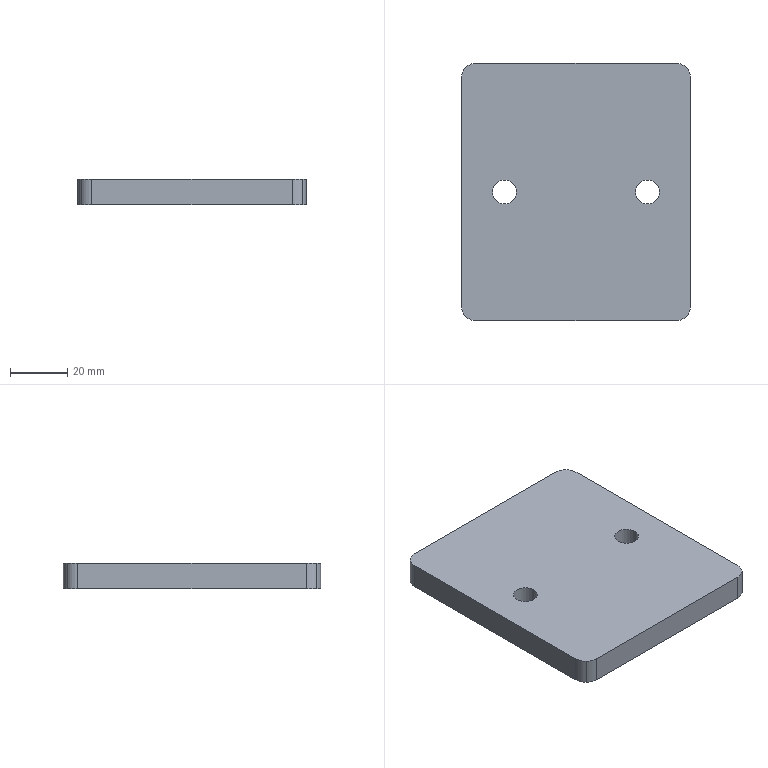Part | STEP file | DCV-000-027 | 1 solid | 18 faces | box 80 x 90 x 9 mm | volume 63615 mm3 | cylinder 12 | plane 6 | commonest cylinder face diameters 10 x8 8.376 x4
STEP:
#1=CARTESIAN_POINT('',(0.,0.,0.));
#2=DIRECTION('',(0.,0.,1.));
#3=DIRECTION('',(1.,0.,0.));
#4=AXIS2_PLACEMENT_3D('',#1,#2,#3);
#5=CARTESIAN_POINT('',(35.,0.,0.));
#6=VERTEX_POINT('',#5);
#7=CARTESIAN_POINT('',(38.536,1.464,0.));
#8=VERTEX_POINT('',#7);
#9=CARTESIAN_POINT('',(35.,5.,0.));
#10=DIRECTION('',(0.,0.,1.));
#11=DIRECTION('',(0.7071,-0.7071,0.));
#12=AXIS2_PLACEMENT_3D('',#9,#10,#11);
#13=CIRCLE('',#12,5.);
#14=CARTESIAN_POINT('',(35.,5.,0.));
#15=DIRECTION('',(0.,0.,1.));
#16=DIRECTION('',(0.7071,-0.7071,0.));
#17=AXIS2_PLACEMENT_3D('',#14,#15,#16);
#18=CYLINDRICAL_SURFACE('',#17,5.);
#19=CARTESIAN_POINT('',(0.,0.));
#20=DIRECTION('',(1.,0.));
#21=VECTOR('',#20,1.);
#22=LINE('',#19,#21);
#23=(GEOMETRIC_REPRESENTATION_CONTEXT(2)PARAMETRIC_REPRESENTATION_CONTEXT()REPRESENTATION_CONTEXT('',''));
#24=DEFINITIONAL_REPRESENTATION('',(#22),#23);
#25=PCURVE('',#18,#24);
#26=CARTESIAN_POINT('',(0.,45.,0.));
#27=DIRECTION('',(0.,0.,1.));
#28=DIRECTION('',(1.,0.,0.));
#29=AXIS2_PLACEMENT_3D('',#26,#27,#28);
#30=PLANE('',#29);
#31=CARTESIAN_POINT('',(35.,-40.));
#32=DIRECTION('',(0.7071,-0.7071));
#33=AXIS2_PLACEMENT_2D('',#31,#32);
#34=CIRCLE('',#33,5.);
#35=(GEOMETRIC_REPRESENTATION_CONTEXT(2)PARAMETRIC_REPRESENTATION_CONTEXT()REPRESENTATION_CONTEXT('',''));
#36=DEFINITIONAL_REPRESENTATION('',(#34),#35);
#37=PCURVE('',#30,#36);
#38=SURFACE_CURVE('',#13,(#25,#37),.PCURVE_S1.);
#39=EDGE_CURVE('',#6,#8,#38,.T.);
#40=ORIENTED_EDGE('',*,*,#39,.T.);
#41=CARTESIAN_POINT('',(38.536,1.464,9.));
#42=VERTEX_POINT('',#41);
#43=CARTESIAN_POINT('',(38.536,1.464,0.));
#44=DIRECTION('',(0.,0.,1.));
#45=VECTOR('',#44,1.);
#46=LINE('',#43,#45);
#47=CARTESIAN_POINT('',(6.283,0.));
#48=DIRECTION('',(0.,1.));
#49=VECTOR('',#48,1.);
#50=LINE('',#47,#49);
#51=(GEOMETRIC_REPRESENTATION_CONTEXT(2)PARAMETRIC_REPRESENTATION_CONTEXT()REPRESENTATION_CONTEXT('',''));
#52=DEFINITIONAL_REPRESENTATION('',(#50),#51);
#53=PCURVE('',#18,#52);
#54=CARTESIAN_POINT('',(35.,5.,0.));
#55=DIRECTION('',(0.,0.,1.));
#56=DIRECTION('',(0.7071,-0.7071,0.));
#57=AXIS2_PLACEMENT_3D('',#54,#55,#56);
#58=CYLINDRICAL_SURFACE('',#57,5.);
#59=CARTESIAN_POINT('',(0.,0.));
#60=DIRECTION('',(0.,1.));
#61=VECTOR('',#60,1.);
#62=LINE('',#59,#61);
#63=(GEOMETRIC_REPRESENTATION_CONTEXT(2)PARAMETRIC_REPRESENTATION_CONTEXT()REPRESENTATION_CONTEXT('',''));
#64=DEFINITIONAL_REPRESENTATION('',(#62),#63);
#65=PCURVE('',#58,#64);
#66=SURFACE_CURVE('',#46,(#53,#65),.PCURVE_S1.);
#67=EDGE_CURVE('',#8,#42,#66,.T.);
#68=ORIENTED_EDGE('',*,*,#67,.T.);
#69=CARTESIAN_POINT('',(35.,0.,9.));
#70=VERTEX_POINT('',#69);
#71=CARTESIAN_POINT('',(35.,5.,9.));
#72=DIRECTION('',(0.,0.,-1.));
#73=DIRECTION('',(0.7071,-0.7071,0.));
#74=AXIS2_PLACEMENT_3D('',#71,#72,#73);
#75=CIRCLE('',#74,5.);
#76=CARTESIAN_POINT('',(6.283,9.));
#77=DIRECTION('',(-1.,0.));
#78=VECTOR('',#77,1.);
#79=LINE('',#76,#78);
#80=(GEOMETRIC_REPRESENTATION_CONTEXT(2)PARAMETRIC_REPRESENTATION_CONTEXT()REPRESENTATION_CONTEXT('',''));
#81=DEFINITIONAL_REPRESENTATION('',(#79),#80);
#82=PCURVE('',#18,#81);
#83=CARTESIAN_POINT('',(0.,45.,9.));
#84=DIRECTION('',(0.,0.,1.));
#85=DIRECTION('',(1.,0.,0.));
#86=AXIS2_PLACEMENT_3D('',#83,#84,#85);
#87=PLANE('',#86);
#88=CARTESIAN_POINT('',(38.536,-43.536));
#89=CARTESIAN_POINT('',(32.412,-49.659));
#90=CARTESIAN_POINT('',(30.17,-41.294));
#91=CARTESIAN_POINT('',(27.929,-32.929));
#92=CARTESIAN_POINT('',(36.294,-35.17));
#93=CARTESIAN_POINT('',(44.659,-37.412));
#94=CARTESIAN_POINT('',(38.536,-43.536));
#95=(BOUNDED_CURVE()B_SPLINE_CURVE(2,(#88,#89,#90,#91,#92,#93,#94),.UNSPECIFIED.,.T.,.F.)B_SPLINE_CURVE_WITH_KNOTS((1,2,2,2,2,1),(-2.094,0.,2.094,4.189,6.283,8.378),.UNSPECIFIED.)CURVE()GEOMETRIC_REPRESENTATION_ITEM()RATIONAL_B_SPLINE_CURVE((1.,0.5,1.,0.5,1.,0.5,1.))REPRESENTATION_ITEM(''));
#96=(GEOMETRIC_REPRESENTATION_CONTEXT(2)PARAMETRIC_REPRESENTATION_CONTEXT()REPRESENTATION_CONTEXT('',''));
#97=DEFINITIONAL_REPRESENTATION('',(#95),#96);
#98=PCURVE('',#87,#97);
#99=SURFACE_CURVE('',#75,(#82,#98),.PCURVE_S1.);
#100=EDGE_CURVE('',#42,#70,#99,.T.);
#101=ORIENTED_EDGE('',*,*,#100,.T.);
#102=CARTESIAN_POINT('',(35.,0.,0.));
#103=DIRECTION('',(0.,0.,-1.));
#104=VECTOR('',#103,1.);
#105=LINE('',#102,#104);
#106=CARTESIAN_POINT('',(5.498,0.));
#107=DIRECTION('',(0.,-1.));
#108=VECTOR('',#107,1.);
#109=LINE('',#106,#108);
#110=(GEOMETRIC_REPRESENTATION_CONTEXT(2)PARAMETRIC_REPRESENTATION_CONTEXT()REPRESENTATION_CONTEXT('',''));
#111=DEFINITIONAL_REPRESENTATION('',(#109),#110);
#112=PCURVE('',#18,#111);
#113=CARTESIAN_POINT('',(-40.,0.,0.));
#114=DIRECTION('',(0.,-1.,0.));
#115=DIRECTION('',(0.,0.,-1.));
#116=AXIS2_PLACEMENT_3D('',#113,#114,#115);
#117=PLANE('',#116);
#118=CARTESIAN_POINT('',(0.,75.));
#119=DIRECTION('',(1.,0.));
#120=VECTOR('',#119,1.);
#121=LINE('',#118,#120);
#122=(GEOMETRIC_REPRESENTATION_CONTEXT(2)PARAMETRIC_REPRESENTATION_CONTEXT()REPRESENTATION_CONTEXT('',''));
#123=DEFINITIONAL_REPRESENTATION('',(#121),#122);
#124=PCURVE('',#117,#123);
#125=SURFACE_CURVE('',#105,(#112,#124),.PCURVE_S1.);
#126=EDGE_CURVE('',#70,#6,#125,.T.);
#127=ORIENTED_EDGE('',*,*,#126,.T.);
#128=EDGE_LOOP('',(#40,#68,#101,#127));
#129=FACE_BOUND('',#128,.T.);
#130=ADVANCED_FACE('',(#129),#18,.T.);
#131=CARTESIAN_POINT('',(-40.,5.,0.));
#132=VERTEX_POINT('',#131);
#133=CARTESIAN_POINT('',(-38.536,1.464,0.));
#134=VERTEX_POINT('',#133);
#135=CARTESIAN_POINT('',(-35.,5.,0.));
#136=DIRECTION('',(0.,0.,1.));
#137=DIRECTION('',(-0.7071,-0.7071,0.));
#138=AXIS2_PLACEMENT_3D('',#135,#136,#137);
#139=CIRCLE('',#138,5.);
#140=CARTESIAN_POINT('',(-35.,5.,0.));
#141=DIRECTION('',(0.,0.,1.));
#142=DIRECTION('',(-0.7071,-0.7071,0.));
#143=AXIS2_PLACEMENT_3D('',#140,#141,#142);
#144=CYLINDRICAL_SURFACE('',#143,5.);
#145=CARTESIAN_POINT('',(0.,0.));
#146=DIRECTION('',(1.,0.));
#147=VECTOR('',#146,1.);
#148=LINE('',#145,#147);
#149=(GEOMETRIC_REPRESENTATION_CONTEXT(2)PARAMETRIC_REPRESENTATION_CONTEXT()REPRESENTATION_CONTEXT('',''));
#150=DEFINITIONAL_REPRESENTATION('',(#148),#149);
#151=PCURVE('',#144,#150);
#152=CARTESIAN_POINT('',(-35.,-40.));
#153=DIRECTION('',(-0.7071,-0.7071));
#154=AXIS2_PLACEMENT_2D('',#152,#153);
#155=CIRCLE('',#154,5.);
#156=(GEOMETRIC_REPRESENTATION_CONTEXT(2)PARAMETRIC_REPRESENTATION_CONTEXT()REPRESENTATION_CONTEXT('',''));
#157=DEFINITIONAL_REPRESENTATION('',(#155),#156);
#158=PCURVE('',#30,#157);
#159=SURFACE_CURVE('',#139,(#151,#158),.PCURVE_S1.);
#160=EDGE_CURVE('',#132,#134,#159,.T.);
#161=ORIENTED_EDGE('',*,*,#160,.T.);
#162=CARTESIAN_POINT('',(-38.536,1.464,9.));
#163=VERTEX_POINT('',#162);
#164=CARTESIAN_POINT('',(-38.536,1.464,0.));
#165=DIRECTION('',(0.,0.,1.));
#166=VECTOR('',#165,1.);
#167=LINE('',#164,#166);
#168=CARTESIAN_POINT('',(6.283,0.));
#169=DIRECTION('',(0.,1.));
#170=VECTOR('',#169,1.);
#171=LINE('',#168,#170);
#172=(GEOMETRIC_REPRESENTATION_CONTEXT(2)PARAMETRIC_REPRESENTATION_CONTEXT()REPRESENTATION_CONTEXT('',''));
#173=DEFINITIONAL_REPRESENTATION('',(#171),#172);
#174=PCURVE('',#144,#173);
#175=CARTESIAN_POINT('',(-35.,5.,0.));
#176=DIRECTION('',(0.,0.,1.));
#177=DIRECTION('',(-0.7071,-0.7071,0.));
#178=AXIS2_PLACEMENT_3D('',#175,#176,#177);
#179=CYLINDRICAL_SURFACE('',#178,5.);
#180=CARTESIAN_POINT('',(0.,0.));
#181=DIRECTION('',(0.,1.));
#182=VECTOR('',#181,1.);
#183=LINE('',#180,#182);
#184=(GEOMETRIC_REPRESENTATION_CONTEXT(2)PARAMETRIC_REPRESENTATION_CONTEXT()REPRESENTATION_CONTEXT('',''));
#185=DEFINITIONAL_REPRESENTATION('',(#183),#184);
#186=PCURVE('',#179,#185);
#187=SURFACE_CURVE('',#167,(#174,#186),.PCURVE_S1.);
#188=EDGE_CURVE('',#134,#163,#187,.T.);
#189=ORIENTED_EDGE('',*,*,#188,.T.);
#190=CARTESIAN_POINT('',(-40.,5.,9.));
#191=VERTEX_POINT('',#190);
#192=CARTESIAN_POINT('',(-35.,5.,9.));
#193=DIRECTION('',(0.,0.,-1.));
#194=DIRECTION('',(-0.7071,-0.7071,0.));
#195=AXIS2_PLACEMENT_3D('',#192,#193,#194);
#196=CIRCLE('',#195,5.);
#197=CARTESIAN_POINT('',(6.283,9.));
#198=DIRECTION('',(-1.,0.));
#199=VECTOR('',#198,1.);
#200=LINE('',#197,#199);
#201=(GEOMETRIC_REPRESENTATION_CONTEXT(2)PARAMETRIC_REPRESENTATION_CONTEXT()REPRESENTATION_CONTEXT('',''));
#202=DEFINITIONAL_REPRESENTATION('',(#200),#201);
#203=PCURVE('',#144,#202);
#204=CARTESIAN_POINT('',(-38.536,-43.536));
#205=CARTESIAN_POINT('',(-44.659,-37.412));
#206=CARTESIAN_POINT('',(-36.294,-35.17));
#207=CARTESIAN_POINT('',(-27.929,-32.929));
#208=CARTESIAN_POINT('',(-30.17,-41.294));
#209=CARTESIAN_POINT('',(-32.412,-49.659));
#210=CARTESIAN_POINT('',(-38.536,-43.536));
#211=(BOUNDED_CURVE()B_SPLINE_CURVE(2,(#204,#205,#206,#207,#208,#209,#210),.UNSPECIFIED.,.T.,.F.)B_SPLINE_CURVE_WITH_KNOTS((1,2,2,2,2,1),(-2.094,0.,2.094,4.189,6.283,8.378),.UNSPECIFIED.)CURVE()GEOMETRIC_REPRESENTATION_ITEM()RATIONAL_B_SPLINE_CURVE((1.,0.5,1.,0.5,1.,0.5,1.))REPRESENTATION_ITEM(''));
#212=(GEOMETRIC_REPRESENTATION_CONTEXT(2)PARAMETRIC_REPRESENTATION_CONTEXT()REPRESENTATION_CONTEXT('',''));
#213=DEFINITIONAL_REPRESENTATION('',(#211),#212);
#214=PCURVE('',#87,#213);
#215=SURFACE_CURVE('',#196,(#203,#214),.PCURVE_S1.);
#216=EDGE_CURVE('',#163,#191,#215,.T.);
#217=ORIENTED_EDGE('',*,*,#216,.T.);
#218=CARTESIAN_POINT('',(-40.,5.,0.));
#219=DIRECTION('',(0.,0.,-1.));
#220=VECTOR('',#219,1.);
#221=LINE('',#218,#220);
#222=CARTESIAN_POINT('',(5.498,0.));
#223=DIRECTION('',(0.,-1.));
#224=VECTOR('',#223,1.);
#225=LINE('',#222,#224);
#226=(GEOMETRIC_REPRESENTATION_CONTEXT(2)PARAMETRIC_REPRESENTATION_CONTEXT()REPRESENTATION_CONTEXT('',''));
#227=DEFINITIONAL_REPRESENTATION('',(#225),#226);
#228=PCURVE('',#144,#227);
#229=CARTESIAN_POINT('',(-40.,90.,0.));
#230=DIRECTION('',(-1.,0.,0.));
#231=DIRECTION('',(0.,0.,1.));
#232=AXIS2_PLACEMENT_3D('',#229,#230,#231);
#233=PLANE('',#232);
#234=CARTESIAN_POINT('',(0.,-85.));
#235=DIRECTION('',(-1.,0.));
#236=VECTOR('',#235,1.);
#237=LINE('',#234,#236);
#238=(GEOMETRIC_REPRESENTATION_CONTEXT(2)PARAMETRIC_REPRESENTATION_CONTEXT()REPRESENTATION_CONTEXT('',''));
#239=DEFINITIONAL_REPRESENTATION('',(#237),#238);
#240=PCURVE('',#233,#239);
#241=SURFACE_CURVE('',#221,(#228,#240),.PCURVE_S1.);
#242=EDGE_CURVE('',#191,#132,#241,.T.);
#243=ORIENTED_EDGE('',*,*,#242,.T.);
#244=EDGE_LOOP('',(#161,#189,#217,#243));
#245=FACE_BOUND('',#244,.T.);
#246=ADVANCED_FACE('',(#245),#144,.T.);
#247=CARTESIAN_POINT('',(-35.,90.,0.));
#248=VERTEX_POINT('',#247);
#249=CARTESIAN_POINT('',(-38.536,88.536,0.));
#250=VERTEX_POINT('',#249);
#251=CARTESIAN_POINT('',(-35.,85.,0.));
#252=DIRECTION('',(0.,0.,1.));
#253=DIRECTION('',(-0.7071,0.7071,0.));
#254=AXIS2_PLACEMENT_3D('',#251,#252,#253);
#255=CIRCLE('',#254,5.);
#256=CARTESIAN_POINT('',(-35.,85.,0.));
#257=DIRECTION('',(0.,0.,1.));
#258=DIRECTION('',(-0.7071,0.7071,0.));
#259=AXIS2_PLACEMENT_3D('',#256,#257,#258);
#260=CYLINDRICAL_SURFACE('',#259,5.);
#261=CARTESIAN_POINT('',(0.,0.));
#262=DIRECTION('',(1.,0.));
#263=VECTOR('',#262,1.);
#264=LINE('',#261,#263);
#265=(GEOMETRIC_REPRESENTATION_CONTEXT(2)PARAMETRIC_REPRESENTATION_CONTEXT()REPRESENTATION_CONTEXT('',''));
#266=DEFINITIONAL_REPRESENTATION('',(#264),#265);
#267=PCURVE('',#260,#266);
#268=CARTESIAN_POINT('',(-35.,40.));
#269=DIRECTION('',(-0.7071,0.7071));
#270=AXIS2_PLACEMENT_2D('',#268,#269);
#271=CIRCLE('',#270,5.);
#272=(GEOMETRIC_REPRESENTATION_CONTEXT(2)PARAMETRIC_REPRESENTATION_CONTEXT()REPRESENTATION_CONTEXT('',''));
#273=DEFINITIONAL_REPRESENTATION('',(#271),#272);
#274=PCURVE('',#30,#273);
#275=SURFACE_CURVE('',#255,(#267,#274),.PCURVE_S1.);
#276=EDGE_CURVE('',#248,#250,#275,.T.);
#277=ORIENTED_EDGE('',*,*,#276,.T.);
#278=CARTESIAN_POINT('',(-38.536,88.536,9.));
#279=VERTEX_POINT('',#278);
#280=CARTESIAN_POINT('',(-38.536,88.536,0.));
#281=DIRECTION('',(0.,0.,1.));
#282=VECTOR('',#281,1.);
#283=LINE('',#280,#282);
#284=CARTESIAN_POINT('',(6.283,0.));
#285=DIRECTION('',(0.,1.));
#286=VECTOR('',#285,1.);
#287=LINE('',#284,#286);
#288=(GEOMETRIC_REPRESENTATION_CONTEXT(2)PARAMETRIC_REPRESENTATION_CONTEXT()REPRESENTATION_CONTEXT('',''));
#289=DEFINITIONAL_REPRESENTATION('',(#287),#288);
#290=PCURVE('',#260,#289);
#291=CARTESIAN_POINT('',(-35.,85.,0.));
#292=DIRECTION('',(0.,0.,1.));
#293=DIRECTION('',(-0.7071,0.7071,0.));
#294=AXIS2_PLACEMENT_3D('',#291,#292,#293);
#295=CYLINDRICAL_SURFACE('',#294,5.);
#296=CARTESIAN_POINT('',(0.,0.));
#297=DIRECTION('',(0.,1.));
#298=VECTOR('',#297,1.);
#299=LINE('',#296,#298);
#300=(GEOMETRIC_REPRESENTATION_CONTEXT(2)PARAMETRIC_REPRESENTATION_CONTEXT()REPRESENTATION_CONTEXT('',''));
#301=DEFINITIONAL_REPRESENTATION('',(#299),#300);
#302=PCURVE('',#295,#301);
#303=SURFACE_CURVE('',#283,(#290,#302),.PCURVE_S1.);
#304=EDGE_CURVE('',#250,#279,#303,.T.);
#305=ORIENTED_EDGE('',*,*,#304,.T.);
#306=CARTESIAN_POINT('',(-35.,90.,9.));
#307=VERTEX_POINT('',#306);
#308=CARTESIAN_POINT('',(-35.,85.,9.));
#309=DIRECTION('',(0.,0.,-1.));
#310=DIRECTION('',(-0.7071,0.7071,0.));
#311=AXIS2_PLACEMENT_3D('',#308,#309,#310);
#312=CIRCLE('',#311,5.);
#313=CARTESIAN_POINT('',(6.283,9.));
#314=DIRECTION('',(-1.,0.));
#315=VECTOR('',#314,1.);
#316=LINE('',#313,#315);
#317=(GEOMETRIC_REPRESENTATION_CONTEXT(2)PARAMETRIC_REPRESENTATION_CONTEXT()REPRESENTATION_CONTEXT('',''));
#318=DEFINITIONAL_REPRESENTATION('',(#316),#317);
#319=PCURVE('',#260,#318);
#320=CARTESIAN_POINT('',(-38.536,43.536));
#321=CARTESIAN_POINT('',(-32.412,49.659));
#322=CARTESIAN_POINT('',(-30.17,41.294));
#323=CARTESIAN_POINT('',(-27.929,32.929));
#324=CARTESIAN_POINT('',(-36.294,35.17));
#325=CARTESIAN_POINT('',(-44.659,37.412));
#326=CARTESIAN_POINT('',(-38.536,43.536));
#327=(BOUNDED_CURVE()B_SPLINE_CURVE(2,(#320,#321,#322,#323,#324,#325,#326),.UNSPECIFIED.,.T.,.F.)B_SPLINE_CURVE_WITH_KNOTS((1,2,2,2,2,1),(-2.094,0.,2.094,4.189,6.283,8.378),.UNSPECIFIED.)CURVE()GEOMETRIC_REPRESENTATION_ITEM()RATIONAL_B_SPLINE_CURVE((1.,0.5,1.,0.5,1.,0.5,1.))REPRESENTATION_ITEM(''));
#328=(GEOMETRIC_REPRESENTATION_CONTEXT(2)PARAMETRIC_REPRESENTATION_CONTEXT()REPRESENTATION_CONTEXT('',''));
#329=DEFINITIONAL_REPRESENTATION('',(#327),#328);
#330=PCURVE('',#87,#329);
#331=SURFACE_CURVE('',#312,(#319,#330),.PCURVE_S1.);
#332=EDGE_CURVE('',#279,#307,#331,.T.);
#333=ORIENTED_EDGE('',*,*,#332,.T.);
#334=CARTESIAN_POINT('',(-35.,90.,0.));
#335=DIRECTION('',(0.,0.,-1.));
#336=VECTOR('',#335,1.);
#337=LINE('',#334,#336);
#338=CARTESIAN_POINT('',(5.498,0.));
#339=DIRECTION('',(0.,-1.));
#340=VECTOR('',#339,1.);
#341=LINE('',#338,#340);
#342=(GEOMETRIC_REPRESENTATION_CONTEXT(2)PARAMETRIC_REPRESENTATION_CONTEXT()REPRESENTATION_CONTEXT('',''));
#343=DEFINITIONAL_REPRESENTATION('',(#341),#342);
#344=PCURVE('',#260,#343);
#345=CARTESIAN_POINT('',(40.,90.,0.));
#346=DIRECTION('',(0.,1.,0.));
#347=DIRECTION('',(1.,0.,0.));
#348=AXIS2_PLACEMENT_3D('',#345,#346,#347);
#349=PLANE('',#348);
#350=CARTESIAN_POINT('',(-75.,0.));
#351=DIRECTION('',(0.,1.));
#352=VECTOR('',#351,1.);
#353=LINE('',#350,#352);
#354=(GEOMETRIC_REPRESENTATION_CONTEXT(2)PARAMETRIC_REPRESENTATION_CONTEXT()REPRESENTATION_CONTEXT('',''));
#355=DEFINITIONAL_REPRESENTATION('',(#353),#354);
#356=PCURVE('',#349,#355);
#357=SURFACE_CURVE('',#337,(#344,#356),.PCURVE_S1.);
#358=EDGE_CURVE('',#307,#248,#357,.T.);
#359=ORIENTED_EDGE('',*,*,#358,.T.);
#360=EDGE_LOOP('',(#277,#305,#333,#359));
#361=FACE_BOUND('',#360,.T.);
#362=ADVANCED_FACE('',(#361),#260,.T.);
#363=CARTESIAN_POINT('',(40.,85.,0.));
#364=VERTEX_POINT('',#363);
#365=CARTESIAN_POINT('',(38.536,88.536,0.));
#366=VERTEX_POINT('',#365);
#367=CARTESIAN_POINT('',(35.,85.,0.));
#368=DIRECTION('',(0.,0.,1.));
#369=DIRECTION('',(0.7071,0.7071,0.));
#370=AXIS2_PLACEMENT_3D('',#367,#368,#369);
#371=CIRCLE('',#370,5.);
#372=CARTESIAN_POINT('',(35.,85.,0.));
#373=DIRECTION('',(0.,0.,1.));
#374=DIRECTION('',(0.7071,0.7071,0.));
#375=AXIS2_PLACEMENT_3D('',#372,#373,#374);
#376=CYLINDRICAL_SURFACE('',#375,5.);
#377=CARTESIAN_POINT('',(0.,0.));
#378=DIRECTION('',(1.,0.));
#379=VECTOR('',#378,1.);
#380=LINE('',#377,#379);
#381=(GEOMETRIC_REPRESENTATION_CONTEXT(2)PARAMETRIC_REPRESENTATION_CONTEXT()REPRESENTATION_CONTEXT('',''));
#382=DEFINITIONAL_REPRESENTATION('',(#380),#381);
#383=PCURVE('',#376,#382);
#384=CARTESIAN_POINT('',(35.,40.));
#385=DIRECTION('',(0.7071,0.7071));
#386=AXIS2_PLACEMENT_2D('',#384,#385);
#387=CIRCLE('',#386,5.);
#388=(GEOMETRIC_REPRESENTATION_CONTEXT(2)PARAMETRIC_REPRESENTATION_CONTEXT()REPRESENTATION_CONTEXT('',''));
#389=DEFINITIONAL_REPRESENTATION('',(#387),#388);
#390=PCURVE('',#30,#389);
#391=SURFACE_CURVE('',#371,(#383,#390),.PCURVE_S1.);
#392=EDGE_CURVE('',#364,#366,#391,.T.);
#393=ORIENTED_EDGE('',*,*,#392,.T.);
#394=CARTESIAN_POINT('',(38.536,88.536,9.));
#395=VERTEX_POINT('',#394);
#396=CARTESIAN_POINT('',(38.536,88.536,0.));
#397=DIRECTION('',(0.,0.,1.));
#398=VECTOR('',#397,1.);
#399=LINE('',#396,#398);
#400=CARTESIAN_POINT('',(6.283,0.));
#401=DIRECTION('',(0.,1.));
#402=VECTOR('',#401,1.);
#403=LINE('',#400,#402);
#404=(GEOMETRIC_REPRESENTATION_CONTEXT(2)PARAMETRIC_REPRESENTATION_CONTEXT()REPRESENTATION_CONTEXT('',''));
#405=DEFINITIONAL_REPRESENTATION('',(#403),#404);
#406=PCURVE('',#376,#405);
#407=CARTESIAN_POINT('',(35.,85.,0.));
#408=DIRECTION('',(0.,0.,1.));
#409=DIRECTION('',(0.7071,0.7071,0.));
#410=AXIS2_PLACEMENT_3D('',#407,#408,#409);
#411=CYLINDRICAL_SURFACE('',#410,5.);
#412=CARTESIAN_POINT('',(0.,0.));
#413=DIRECTION('',(0.,1.));
#414=VECTOR('',#413,1.);
#415=LINE('',#412,#414);
#416=(GEOMETRIC_REPRESENTATION_CONTEXT(2)PARAMETRIC_REPRESENTATION_CONTEXT()REPRESENTATION_CONTEXT('',''));
#417=DEFINITIONAL_REPRESENTATION('',(#415),#416);
#418=PCURVE('',#411,#417);
#419=SURFACE_CURVE('',#399,(#406,#418),.PCURVE_S1.);
#420=EDGE_CURVE('',#366,#395,#419,.T.);
#421=ORIENTED_EDGE('',*,*,#420,.T.);
#422=CARTESIAN_POINT('',(40.,85.,9.));
#423=VERTEX_POINT('',#422);
#424=CARTESIAN_POINT('',(35.,85.,9.));
#425=DIRECTION('',(0.,0.,-1.));
#426=DIRECTION('',(0.7071,0.7071,0.));
#427=AXIS2_PLACEMENT_3D('',#424,#425,#426);
#428=CIRCLE('',#427,5.);
#429=CARTESIAN_POINT('',(6.283,9.));
#430=DIRECTION('',(-1.,0.));
#431=VECTOR('',#430,1.);
#432=LINE('',#429,#431);
#433=(GEOMETRIC_REPRESENTATION_CONTEXT(2)PARAMETRIC_REPRESENTATION_CONTEXT()REPRESENTATION_CONTEXT('',''));
#434=DEFINITIONAL_REPRESENTATION('',(#432),#433);
#435=PCURVE('',#376,#434);
#436=CARTESIAN_POINT('',(38.536,43.536));
#437=CARTESIAN_POINT('',(44.659,37.412));
#438=CARTESIAN_POINT('',(36.294,35.17));
#439=CARTESIAN_POINT('',(27.929,32.929));
#440=CARTESIAN_POINT('',(30.17,41.294));
#441=CARTESIAN_POINT('',(32.412,49.659));
#442=CARTESIAN_POINT('',(38.536,43.536));
#443=(BOUNDED_CURVE()B_SPLINE_CURVE(2,(#436,#437,#438,#439,#440,#441,#442),.UNSPECIFIED.,.T.,.F.)B_SPLINE_CURVE_WITH_KNOTS((1,2,2,2,2,1),(-2.094,0.,2.094,4.189,6.283,8.378),.UNSPECIFIED.)CURVE()GEOMETRIC_REPRESENTATION_ITEM()RATIONAL_B_SPLINE_CURVE((1.,0.5,1.,0.5,1.,0.5,1.))REPRESENTATION_ITEM(''));
#444=(GEOMETRIC_REPRESENTATION_CONTEXT(2)PARAMETRIC_REPRESENTATION_CONTEXT()REPRESENTATION_CONTEXT('',''));
#445=DEFINITIONAL_REPRESENTATION('',(#443),#444);
#446=PCURVE('',#87,#445);
#447=SURFACE_CURVE('',#428,(#435,#446),.PCURVE_S1.);
#448=EDGE_CURVE('',#395,#423,#447,.T.);
#449=ORIENTED_EDGE('',*,*,#448,.T.);
#450=CARTESIAN_POINT('',(40.,85.,0.));
#451=DIRECTION('',(0.,0.,-1.));
#452=VECTOR('',#451,1.);
#453=LINE('',#450,#452);
#454=CARTESIAN_POINT('',(5.498,0.));
#455=DIRECTION('',(0.,-1.));
#456=VECTOR('',#455,1.);
#457=LINE('',#454,#456);
#458=(GEOMETRIC_REPRESENTATION_CONTEXT(2)PARAMETRIC_REPRESENTATION_CONTEXT()REPRESENTATION_CONTEXT('',''));
#459=DEFINITIONAL_REPRESENTATION('',(#457),#458);
#460=PCURVE('',#376,#459);
#461=CARTESIAN_POINT('',(40.,0.,0.));
#462=DIRECTION('',(1.,0.,0.));
#463=DIRECTION('',(0.,1.,0.));
#464=AXIS2_PLACEMENT_3D('',#461,#462,#463);
#465=PLANE('',#464);
#466=CARTESIAN_POINT('',(85.,0.));
#467=DIRECTION('',(0.,-1.));
#468=VECTOR('',#467,1.);
#469=LINE('',#466,#468);
#470=(GEOMETRIC_REPRESENTATION_CONTEXT(2)PARAMETRIC_REPRESENTATION_CONTEXT()REPRESENTATION_CONTEXT('',''));
#471=DEFINITIONAL_REPRESENTATION('',(#469),#470);
#472=PCURVE('',#465,#471);
#473=SURFACE_CURVE('',#453,(#460,#472),.PCURVE_S1.);
#474=EDGE_CURVE('',#423,#364,#473,.T.);
#475=ORIENTED_EDGE('',*,*,#474,.T.);
#476=EDGE_LOOP('',(#393,#421,#449,#475));
#477=FACE_BOUND('',#476,.T.);
#478=ADVANCED_FACE('',(#477),#376,.T.);
#479=CARTESIAN_POINT('',(29.188,45.,0.));
#480=VERTEX_POINT('',#479);
#481=CARTESIAN_POINT('',(29.188,45.,9.));
#482=VERTEX_POINT('',#481);
#483=CARTESIAN_POINT('',(29.188,45.,-111.752));
#484=DIRECTION('',(0.,0.,1.));
#485=VECTOR('',#484,1.);
#486=LINE('',#483,#485);
#487=CARTESIAN_POINT('',(25.,45.,-111.752));
#488=DIRECTION('',(0.,0.,1.));
#489=DIRECTION('',(1.,0.,0.));
#490=AXIS2_PLACEMENT_3D('',#487,#488,#489);
#491=CYLINDRICAL_SURFACE('',#490,4.188);
#492=CARTESIAN_POINT('',(6.283,0.));
#493=DIRECTION('',(0.,1.));
#494=VECTOR('',#493,1.);
#495=LINE('',#492,#494);
#496=(GEOMETRIC_REPRESENTATION_CONTEXT(2)PARAMETRIC_REPRESENTATION_CONTEXT()REPRESENTATION_CONTEXT('',''));
#497=DEFINITIONAL_REPRESENTATION('',(#495),#496);
#498=PCURVE('',#491,#497);
#499=CARTESIAN_POINT('',(25.,45.,-111.752));
#500=DIRECTION('',(0.,0.,1.));
#501=DIRECTION('',(1.,0.,0.));
#502=AXIS2_PLACEMENT_3D('',#499,#500,#501);
#503=CYLINDRICAL_SURFACE('',#502,4.188);
#504=CARTESIAN_POINT('',(0.,0.));
#505=DIRECTION('',(0.,1.));
#506=VECTOR('',#505,1.);
#507=LINE('',#504,#506);
#508=(GEOMETRIC_REPRESENTATION_CONTEXT(2)PARAMETRIC_REPRESENTATION_CONTEXT()REPRESENTATION_CONTEXT('',''));
#509=DEFINITIONAL_REPRESENTATION('',(#507),#508);
#510=PCURVE('',#503,#509);
#511=SURFACE_CURVE('',#486,(#498,#510),.PCURVE_S1.);
#512=EDGE_CURVE('',#480,#482,#511,.T.);
#513=ORIENTED_EDGE('',*,*,#512,.T.);
#514=CARTESIAN_POINT('',(20.812,45.,9.));
#515=VERTEX_POINT('',#514);
#516=CARTESIAN_POINT('',(25.,45.,9.));
#517=DIRECTION('',(0.,0.,-1.));
#518=DIRECTION('',(1.,0.,0.));
#519=AXIS2_PLACEMENT_3D('',#516,#517,#518);
#520=CIRCLE('',#519,4.188);
#521=CARTESIAN_POINT('',(6.283,120.752));
#522=DIRECTION('',(-1.,0.));
#523=VECTOR('',#522,1.);
#524=LINE('',#521,#523);
#525=(GEOMETRIC_REPRESENTATION_CONTEXT(2)PARAMETRIC_REPRESENTATION_CONTEXT()REPRESENTATION_CONTEXT('',''));
#526=DEFINITIONAL_REPRESENTATION('',(#524),#525);
#527=PCURVE('',#491,#526);
#528=CARTESIAN_POINT('',(29.188,0.));
#529=CARTESIAN_POINT('',(29.188,-7.254));
#530=CARTESIAN_POINT('',(22.906,-3.627));
#531=CARTESIAN_POINT('',(16.624,0.));
#532=CARTESIAN_POINT('',(22.906,3.627));
#533=CARTESIAN_POINT('',(29.188,7.254));
#534=CARTESIAN_POINT('',(29.188,0.));
#535=(BOUNDED_CURVE()B_SPLINE_CURVE(2,(#528,#529,#530,#531,#532,#533,#534),.UNSPECIFIED.,.T.,.F.)B_SPLINE_CURVE_WITH_KNOTS((1,2,2,2,2,1),(-2.094,0.,2.094,4.189,6.283,8.378),.UNSPECIFIED.)CURVE()GEOMETRIC_REPRESENTATION_ITEM()RATIONAL_B_SPLINE_CURVE((1.,0.5,1.,0.5,1.,0.5,1.))REPRESENTATION_ITEM(''));
#536=(GEOMETRIC_REPRESENTATION_CONTEXT(2)PARAMETRIC_REPRESENTATION_CONTEXT()REPRESENTATION_CONTEXT('',''));
#537=DEFINITIONAL_REPRESENTATION('',(#535),#536);
#538=PCURVE('',#87,#537);
#539=SURFACE_CURVE('',#520,(#527,#538),.PCURVE_S1.);
#540=EDGE_CURVE('',#482,#515,#539,.T.);
#541=ORIENTED_EDGE('',*,*,#540,.T.);
#542=CARTESIAN_POINT('',(20.812,45.,0.));
#543=VERTEX_POINT('',#542);
#544=CARTESIAN_POINT('',(20.812,45.,-111.752));
#545=DIRECTION('',(0.,0.,1.));
#546=VECTOR('',#545,1.);
#547=LINE('',#544,#546);
#548=CARTESIAN_POINT('',(3.142,0.));
#549=DIRECTION('',(0.,1.));
#550=VECTOR('',#549,1.);
#551=LINE('',#548,#550);
#552=(GEOMETRIC_REPRESENTATION_CONTEXT(2)PARAMETRIC_REPRESENTATION_CONTEXT()REPRESENTATION_CONTEXT('',''));
#553=DEFINITIONAL_REPRESENTATION('',(#551),#552);
#554=PCURVE('',#491,#553);
#555=CARTESIAN_POINT('',(3.142,0.));
#556=DIRECTION('',(0.,1.));
#557=VECTOR('',#556,1.);
#558=LINE('',#555,#557);
#559=(GEOMETRIC_REPRESENTATION_CONTEXT(2)PARAMETRIC_REPRESENTATION_CONTEXT()REPRESENTATION_CONTEXT('',''));
#560=DEFINITIONAL_REPRESENTATION('',(#558),#559);
#561=PCURVE('',#503,#560);
#562=SURFACE_CURVE('',#547,(#554,#561),.PCURVE_S1.);
#563=EDGE_CURVE('',#543,#515,#562,.T.);
#564=ORIENTED_EDGE('',*,*,#563,.F.);
#565=CARTESIAN_POINT('',(25.,45.,0.));
#566=DIRECTION('',(0.,0.,1.));
#567=DIRECTION('',(1.,0.,0.));
#568=AXIS2_PLACEMENT_3D('',#565,#566,#567);
#569=CIRCLE('',#568,4.188);
#570=CARTESIAN_POINT('',(0.,111.752));
#571=DIRECTION('',(1.,0.));
#572=VECTOR('',#571,1.);
#573=LINE('',#570,#572);
#574=(GEOMETRIC_REPRESENTATION_CONTEXT(2)PARAMETRIC_REPRESENTATION_CONTEXT()REPRESENTATION_CONTEXT('',''));
#575=DEFINITIONAL_REPRESENTATION('',(#573),#574);
#576=PCURVE('',#491,#575);
#577=CARTESIAN_POINT('',(25.,0.));
#578=DIRECTION('',(1.,0.));
#579=AXIS2_PLACEMENT_2D('',#577,#578);
#580=CIRCLE('',#579,4.188);
#581=(GEOMETRIC_REPRESENTATION_CONTEXT(2)PARAMETRIC_REPRESENTATION_CONTEXT()REPRESENTATION_CONTEXT('',''));
#582=DEFINITIONAL_REPRESENTATION('',(#580),#581);
#583=PCURVE('',#30,#582);
#584=SURFACE_CURVE('',#569,(#576,#583),.PCURVE_S1.);
#585=EDGE_CURVE('',#543,#480,#584,.T.);
#586=ORIENTED_EDGE('',*,*,#585,.T.);
#587=EDGE_LOOP('',(#513,#541,#564,#586));
#588=FACE_BOUND('',#587,.F.);
#589=ADVANCED_FACE('',(#588),#491,.F.);
#590=CARTESIAN_POINT('',(-20.812,45.,0.));
#591=VERTEX_POINT('',#590);
#592=CARTESIAN_POINT('',(-20.812,45.,9.));
#593=VERTEX_POINT('',#592);
#594=CARTESIAN_POINT('',(-20.812,45.,-111.752));
#595=DIRECTION('',(0.,0.,1.));
#596=VECTOR('',#595,1.);
#597=LINE('',#594,#596);
#598=CARTESIAN_POINT('',(-25.,45.,-111.752));
#599=DIRECTION('',(0.,0.,1.));
#600=DIRECTION('',(1.,0.,0.));
#601=AXIS2_PLACEMENT_3D('',#598,#599,#600);
#602=CYLINDRICAL_SURFACE('',#601,4.188);
#603=CARTESIAN_POINT('',(6.283,0.));
#604=DIRECTION('',(0.,1.));
#605=VECTOR('',#604,1.);
#606=LINE('',#603,#605);
#607=(GEOMETRIC_REPRESENTATION_CONTEXT(2)PARAMETRIC_REPRESENTATION_CONTEXT()REPRESENTATION_CONTEXT('',''));
#608=DEFINITIONAL_REPRESENTATION('',(#606),#607);
#609=PCURVE('',#602,#608);
#610=CARTESIAN_POINT('',(-25.,45.,-111.752));
#611=DIRECTION('',(0.,0.,1.));
#612=DIRECTION('',(1.,0.,0.));
#613=AXIS2_PLACEMENT_3D('',#610,#611,#612);
#614=CYLINDRICAL_SURFACE('',#613,4.188);
#615=CARTESIAN_POINT('',(0.,0.));
#616=DIRECTION('',(0.,1.));
#617=VECTOR('',#616,1.);
#618=LINE('',#615,#617);
#619=(GEOMETRIC_REPRESENTATION_CONTEXT(2)PARAMETRIC_REPRESENTATION_CONTEXT()REPRESENTATION_CONTEXT('',''));
#620=DEFINITIONAL_REPRESENTATION('',(#618),#619);
#621=PCURVE('',#614,#620);
#622=SURFACE_CURVE('',#597,(#609,#621),.PCURVE_S1.);
#623=EDGE_CURVE('',#591,#593,#622,.T.);
#624=ORIENTED_EDGE('',*,*,#623,.T.);
#625=CARTESIAN_POINT('',(-29.188,45.,9.));
#626=VERTEX_POINT('',#625);
#627=CARTESIAN_POINT('',(-25.,45.,9.));
#628=DIRECTION('',(0.,0.,-1.));
#629=DIRECTION('',(1.,0.,0.));
#630=AXIS2_PLACEMENT_3D('',#627,#628,#629);
#631=CIRCLE('',#630,4.188);
#632=CARTESIAN_POINT('',(6.283,120.752));
#633=DIRECTION('',(-1.,0.));
#634=VECTOR('',#633,1.);
#635=LINE('',#632,#634);
#636=(GEOMETRIC_REPRESENTATION_CONTEXT(2)PARAMETRIC_REPRESENTATION_CONTEXT()REPRESENTATION_CONTEXT('',''));
#637=DEFINITIONAL_REPRESENTATION('',(#635),#636);
#638=PCURVE('',#602,#637);
#639=CARTESIAN_POINT('',(-20.812,0.));
#640=CARTESIAN_POINT('',(-20.812,-7.254));
#641=CARTESIAN_POINT('',(-27.094,-3.627));
#642=CARTESIAN_POINT('',(-33.376,0.));
#643=CARTESIAN_POINT('',(-27.094,3.627));
#644=CARTESIAN_POINT('',(-20.812,7.254));
#645=CARTESIAN_POINT('',(-20.812,0.));
#646=(BOUNDED_CURVE()B_SPLINE_CURVE(2,(#639,#640,#641,#642,#643,#644,#645),.UNSPECIFIED.,.T.,.F.)B_SPLINE_CURVE_WITH_KNOTS((1,2,2,2,2,1),(-2.094,0.,2.094,4.189,6.283,8.378),.UNSPECIFIED.)CURVE()GEOMETRIC_REPRESENTATION_ITEM()RATIONAL_B_SPLINE_CURVE((1.,0.5,1.,0.5,1.,0.5,1.))REPRESENTATION_ITEM(''));
#647=(GEOMETRIC_REPRESENTATION_CONTEXT(2)PARAMETRIC_REPRESENTATION_CONTEXT()REPRESENTATION_CONTEXT('',''));
#648=DEFINITIONAL_REPRESENTATION('',(#646),#647);
#649=PCURVE('',#87,#648);
#650=SURFACE_CURVE('',#631,(#638,#649),.PCURVE_S1.);
#651=EDGE_CURVE('',#593,#626,#650,.T.);
#652=ORIENTED_EDGE('',*,*,#651,.T.);
#653=CARTESIAN_POINT('',(-29.188,45.,0.));
#654=VERTEX_POINT('',#653);
#655=CARTESIAN_POINT('',(-29.188,45.,-111.752));
#656=DIRECTION('',(0.,0.,1.));
#657=VECTOR('',#656,1.);
#658=LINE('',#655,#657);
#659=CARTESIAN_POINT('',(3.142,0.));
#660=DIRECTION('',(0.,1.));
#661=VECTOR('',#660,1.);
#662=LINE('',#659,#661);
#663=(GEOMETRIC_REPRESENTATION_CONTEXT(2)PARAMETRIC_REPRESENTATION_CONTEXT()REPRESENTATION_CONTEXT('',''));
#664=DEFINITIONAL_REPRESENTATION('',(#662),#663);
#665=PCURVE('',#602,#664);
#666=CARTESIAN_POINT('',(3.142,0.));
#667=DIRECTION('',(0.,1.));
#668=VECTOR('',#667,1.);
#669=LINE('',#666,#668);
#670=(GEOMETRIC_REPRESENTATION_CONTEXT(2)PARAMETRIC_REPRESENTATION_CONTEXT()REPRESENTATION_CONTEXT('',''));
#671=DEFINITIONAL_REPRESENTATION('',(#669),#670);
#672=PCURVE('',#614,#671);
#673=SURFACE_CURVE('',#658,(#665,#672),.PCURVE_S1.);
#674=EDGE_CURVE('',#654,#626,#673,.T.);
#675=ORIENTED_EDGE('',*,*,#674,.F.);
#676=CARTESIAN_POINT('',(-25.,45.,0.));
#677=DIRECTION('',(0.,0.,1.));
#678=DIRECTION('',(1.,0.,0.));
#679=AXIS2_PLACEMENT_3D('',#676,#677,#678);
#680=CIRCLE('',#679,4.188);
#681=CARTESIAN_POINT('',(0.,111.752));
#682=DIRECTION('',(1.,0.));
#683=VECTOR('',#682,1.);
#684=LINE('',#681,#683);
#685=(GEOMETRIC_REPRESENTATION_CONTEXT(2)PARAMETRIC_REPRESENTATION_CONTEXT()REPRESENTATION_CONTEXT('',''));
#686=DEFINITIONAL_REPRESENTATION('',(#684),#685);
#687=PCURVE('',#602,#686);
#688=CARTESIAN_POINT('',(-25.,0.));
#689=DIRECTION('',(1.,0.));
#690=AXIS2_PLACEMENT_2D('',#688,#689);
#691=CIRCLE('',#690,4.188);
#692=(GEOMETRIC_REPRESENTATION_CONTEXT(2)PARAMETRIC_REPRESENTATION_CONTEXT()REPRESENTATION_CONTEXT('',''));
#693=DEFINITIONAL_REPRESENTATION('',(#691),#692);
#694=PCURVE('',#30,#693);
#695=SURFACE_CURVE('',#680,(#687,#694),.PCURVE_S1.);
#696=EDGE_CURVE('',#654,#591,#695,.T.);
#697=ORIENTED_EDGE('',*,*,#696,.T.);
#698=EDGE_LOOP('',(#624,#652,#675,#697));
#699=FACE_BOUND('',#698,.F.);
#700=ADVANCED_FACE('',(#699),#602,.F.);
#701=ORIENTED_EDGE('',*,*,#651,.T.);
#702=CARTESIAN_POINT('',(-25.,45.,9.));
#703=DIRECTION('',(0.,0.,-1.));
#704=DIRECTION('',(1.,0.,0.));
#705=AXIS2_PLACEMENT_3D('',#702,#703,#704);
#706=CIRCLE('',#705,4.188);
#707=CARTESIAN_POINT('',(-20.812,0.));
#708=CARTESIAN_POINT('',(-20.812,-7.254));
#709=CARTESIAN_POINT('',(-27.094,-3.627));
#710=CARTESIAN_POINT('',(-33.376,0.));
#711=CARTESIAN_POINT('',(-27.094,3.627));
#712=CARTESIAN_POINT('',(-20.812,7.254));
#713=CARTESIAN_POINT('',(-20.812,0.));
#714=(BOUNDED_CURVE()B_SPLINE_CURVE(2,(#707,#708,#709,#710,#711,#712,#713),.UNSPECIFIED.,.T.,.F.)B_SPLINE_CURVE_WITH_KNOTS((1,2,2,2,2,1),(-2.094,0.,2.094,4.189,6.283,8.378),.UNSPECIFIED.)CURVE()GEOMETRIC_REPRESENTATION_ITEM()RATIONAL_B_SPLINE_CURVE((1.,0.5,1.,0.5,1.,0.5,1.))REPRESENTATION_ITEM(''));
#715=(GEOMETRIC_REPRESENTATION_CONTEXT(2)PARAMETRIC_REPRESENTATION_CONTEXT()REPRESENTATION_CONTEXT('',''));
#716=DEFINITIONAL_REPRESENTATION('',(#714),#715);
#717=PCURVE('',#87,#716);
#718=CARTESIAN_POINT('',(6.283,120.752));
#719=DIRECTION('',(-1.,0.));
#720=VECTOR('',#719,1.);
#721=LINE('',#718,#720);
#722=(GEOMETRIC_REPRESENTATION_CONTEXT(2)PARAMETRIC_REPRESENTATION_CONTEXT()REPRESENTATION_CONTEXT('',''));
#723=DEFINITIONAL_REPRESENTATION('',(#721),#722);
#724=PCURVE('',#614,#723);
#725=SURFACE_CURVE('',#706,(#717,#724),.PCURVE_S1.);
#726=EDGE_CURVE('',#626,#593,#725,.T.);
#727=ORIENTED_EDGE('',*,*,#726,.T.);
#728=EDGE_LOOP('',(#701,#727));
#729=FACE_BOUND('',#728,.T.);
#730=ORIENTED_EDGE('',*,*,#540,.T.);
#731=CARTESIAN_POINT('',(25.,45.,9.));
#732=DIRECTION('',(0.,0.,-1.));
#733=DIRECTION('',(1.,0.,0.));
#734=AXIS2_PLACEMENT_3D('',#731,#732,#733);
#735=CIRCLE('',#734,4.188);
#736=CARTESIAN_POINT('',(29.188,0.));
#737=CARTESIAN_POINT('',(29.188,-7.254));
#738=CARTESIAN_POINT('',(22.906,-3.627));
#739=CARTESIAN_POINT('',(16.624,0.));
#740=CARTESIAN_POINT('',(22.906,3.627));
#741=CARTESIAN_POINT('',(29.188,7.254));
#742=CARTESIAN_POINT('',(29.188,0.));
#743=(BOUNDED_CURVE()B_SPLINE_CURVE(2,(#736,#737,#738,#739,#740,#741,#742),.UNSPECIFIED.,.T.,.F.)B_SPLINE_CURVE_WITH_KNOTS((1,2,2,2,2,1),(-2.094,0.,2.094,4.189,6.283,8.378),.UNSPECIFIED.)CURVE()GEOMETRIC_REPRESENTATION_ITEM()RATIONAL_B_SPLINE_CURVE((1.,0.5,1.,0.5,1.,0.5,1.))REPRESENTATION_ITEM(''));
#744=(GEOMETRIC_REPRESENTATION_CONTEXT(2)PARAMETRIC_REPRESENTATION_CONTEXT()REPRESENTATION_CONTEXT('',''));
#745=DEFINITIONAL_REPRESENTATION('',(#743),#744);
#746=PCURVE('',#87,#745);
#747=CARTESIAN_POINT('',(6.283,120.752));
#748=DIRECTION('',(-1.,0.));
#749=VECTOR('',#748,1.);
#750=LINE('',#747,#749);
#751=(GEOMETRIC_REPRESENTATION_CONTEXT(2)PARAMETRIC_REPRESENTATION_CONTEXT()REPRESENTATION_CONTEXT('',''));
#752=DEFINITIONAL_REPRESENTATION('',(#750),#751);
#753=PCURVE('',#503,#752);
#754=SURFACE_CURVE('',#735,(#746,#753),.PCURVE_S1.);
#755=EDGE_CURVE('',#515,#482,#754,.T.);
#756=ORIENTED_EDGE('',*,*,#755,.T.);
#757=EDGE_LOOP('',(#730,#756));
#758=FACE_BOUND('',#757,.T.);
#759=CARTESIAN_POINT('',(40.,5.,9.));
#760=VERTEX_POINT('',#759);
#761=CARTESIAN_POINT('',(35.,5.,9.));
#762=DIRECTION('',(0.,0.,-1.));
#763=DIRECTION('',(0.7071,-0.7071,0.));
#764=AXIS2_PLACEMENT_3D('',#761,#762,#763);
#765=CIRCLE('',#764,5.);
#766=CARTESIAN_POINT('',(38.536,-43.536));
#767=CARTESIAN_POINT('',(32.412,-49.659));
#768=CARTESIAN_POINT('',(30.17,-41.294));
#769=CARTESIAN_POINT('',(27.929,-32.929));
#770=CARTESIAN_POINT('',(36.294,-35.17));
#771=CARTESIAN_POINT('',(44.659,-37.412));
#772=CARTESIAN_POINT('',(38.536,-43.536));
#773=(BOUNDED_CURVE()B_SPLINE_CURVE(2,(#766,#767,#768,#769,#770,#771,#772),.UNSPECIFIED.,.T.,.F.)B_SPLINE_CURVE_WITH_KNOTS((1,2,2,2,2,1),(-2.094,0.,2.094,4.189,6.283,8.378),.UNSPECIFIED.)CURVE()GEOMETRIC_REPRESENTATION_ITEM()RATIONAL_B_SPLINE_CURVE((1.,0.5,1.,0.5,1.,0.5,1.))REPRESENTATION_ITEM(''));
#774=(GEOMETRIC_REPRESENTATION_CONTEXT(2)PARAMETRIC_REPRESENTATION_CONTEXT()REPRESENTATION_CONTEXT('',''));
#775=DEFINITIONAL_REPRESENTATION('',(#773),#774);
#776=PCURVE('',#87,#775);
#777=CARTESIAN_POINT('',(6.283,9.));
#778=DIRECTION('',(-1.,0.));
#779=VECTOR('',#778,1.);
#780=LINE('',#777,#779);
#781=(GEOMETRIC_REPRESENTATION_CONTEXT(2)PARAMETRIC_REPRESENTATION_CONTEXT()REPRESENTATION_CONTEXT('',''));
#782=DEFINITIONAL_REPRESENTATION('',(#780),#781);
#783=PCURVE('',#58,#782);
#784=SURFACE_CURVE('',#765,(#776,#783),.PCURVE_S1.);
#785=EDGE_CURVE('',#760,#42,#784,.T.);
#786=ORIENTED_EDGE('',*,*,#785,.F.);
#787=CARTESIAN_POINT('',(40.,0.,9.));
#788=DIRECTION('',(0.,1.,0.));
#789=VECTOR('',#788,1.);
#790=LINE('',#787,#789);
#791=CARTESIAN_POINT('',(40.,-45.));
#792=DIRECTION('',(0.,1.));
#793=VECTOR('',#792,1.);
#794=LINE('',#791,#793);
#795=(GEOMETRIC_REPRESENTATION_CONTEXT(2)PARAMETRIC_REPRESENTATION_CONTEXT()REPRESENTATION_CONTEXT('',''));
#796=DEFINITIONAL_REPRESENTATION('',(#794),#795);
#797=PCURVE('',#87,#796);
#798=CARTESIAN_POINT('',(0.,9.));
#799=DIRECTION('',(1.,0.));
#800=VECTOR('',#799,1.);
#801=LINE('',#798,#800);
#802=(GEOMETRIC_REPRESENTATION_CONTEXT(2)PARAMETRIC_REPRESENTATION_CONTEXT()REPRESENTATION_CONTEXT('',''));
#803=DEFINITIONAL_REPRESENTATION('',(#801),#802);
#804=PCURVE('',#465,#803);
#805=SURFACE_CURVE('',#790,(#797,#804),.PCURVE_S1.);
#806=EDGE_CURVE('',#760,#423,#805,.T.);
#807=ORIENTED_EDGE('',*,*,#806,.T.);
#808=ORIENTED_EDGE('',*,*,#448,.F.);
#809=CARTESIAN_POINT('',(35.,90.,9.));
#810=VERTEX_POINT('',#809);
#811=CARTESIAN_POINT('',(35.,85.,9.));
#812=DIRECTION('',(0.,0.,-1.));
#813=DIRECTION('',(0.7071,0.7071,0.));
#814=AXIS2_PLACEMENT_3D('',#811,#812,#813);
#815=CIRCLE('',#814,5.);
#816=CARTESIAN_POINT('',(38.536,43.536));
#817=CARTESIAN_POINT('',(44.659,37.412));
#818=CARTESIAN_POINT('',(36.294,35.17));
#819=CARTESIAN_POINT('',(27.929,32.929));
#820=CARTESIAN_POINT('',(30.17,41.294));
#821=CARTESIAN_POINT('',(32.412,49.659));
#822=CARTESIAN_POINT('',(38.536,43.536));
#823=(BOUNDED_CURVE()B_SPLINE_CURVE(2,(#816,#817,#818,#819,#820,#821,#822),.UNSPECIFIED.,.T.,.F.)B_SPLINE_CURVE_WITH_KNOTS((1,2,2,2,2,1),(-2.094,0.,2.094,4.189,6.283,8.378),.UNSPECIFIED.)CURVE()GEOMETRIC_REPRESENTATION_ITEM()RATIONAL_B_SPLINE_CURVE((1.,0.5,1.,0.5,1.,0.5,1.))REPRESENTATION_ITEM(''));
#824=(GEOMETRIC_REPRESENTATION_CONTEXT(2)PARAMETRIC_REPRESENTATION_CONTEXT()REPRESENTATION_CONTEXT('',''));
#825=DEFINITIONAL_REPRESENTATION('',(#823),#824);
#826=PCURVE('',#87,#825);
#827=CARTESIAN_POINT('',(6.283,9.));
#828=DIRECTION('',(-1.,0.));
#829=VECTOR('',#828,1.);
#830=LINE('',#827,#829);
#831=(GEOMETRIC_REPRESENTATION_CONTEXT(2)PARAMETRIC_REPRESENTATION_CONTEXT()REPRESENTATION_CONTEXT('',''));
#832=DEFINITIONAL_REPRESENTATION('',(#830),#831);
#833=PCURVE('',#411,#832);
#834=SURFACE_CURVE('',#815,(#826,#833),.PCURVE_S1.);
#835=EDGE_CURVE('',#810,#395,#834,.T.);
#836=ORIENTED_EDGE('',*,*,#835,.F.);
#837=CARTESIAN_POINT('',(40.,90.,9.));
#838=DIRECTION('',(-1.,0.,0.));
#839=VECTOR('',#838,1.);
#840=LINE('',#837,#839);
#841=CARTESIAN_POINT('',(40.,45.));
#842=DIRECTION('',(-1.,0.));
#843=VECTOR('',#842,1.);
#844=LINE('',#841,#843);
#845=(GEOMETRIC_REPRESENTATION_CONTEXT(2)PARAMETRIC_REPRESENTATION_CONTEXT()REPRESENTATION_CONTEXT('',''));
#846=DEFINITIONAL_REPRESENTATION('',(#844),#845);
#847=PCURVE('',#87,#846);
#848=CARTESIAN_POINT('',(0.,-9.));
#849=DIRECTION('',(-1.,0.));
#850=VECTOR('',#849,1.);
#851=LINE('',#848,#850);
#852=(GEOMETRIC_REPRESENTATION_CONTEXT(2)PARAMETRIC_REPRESENTATION_CONTEXT()REPRESENTATION_CONTEXT('',''));
#853=DEFINITIONAL_REPRESENTATION('',(#851),#852);
#854=PCURVE('',#349,#853);
#855=SURFACE_CURVE('',#840,(#847,#854),.PCURVE_S1.);
#856=EDGE_CURVE('',#810,#307,#855,.T.);
#857=ORIENTED_EDGE('',*,*,#856,.T.);
#858=ORIENTED_EDGE('',*,*,#332,.F.);
#859=CARTESIAN_POINT('',(-40.,85.,9.));
#860=VERTEX_POINT('',#859);
#861=CARTESIAN_POINT('',(-35.,85.,9.));
#862=DIRECTION('',(0.,0.,-1.));
#863=DIRECTION('',(-0.7071,0.7071,0.));
#864=AXIS2_PLACEMENT_3D('',#861,#862,#863);
#865=CIRCLE('',#864,5.);
#866=CARTESIAN_POINT('',(-38.536,43.536));
#867=CARTESIAN_POINT('',(-32.412,49.659));
#868=CARTESIAN_POINT('',(-30.17,41.294));
#869=CARTESIAN_POINT('',(-27.929,32.929));
#870=CARTESIAN_POINT('',(-36.294,35.17));
#871=CARTESIAN_POINT('',(-44.659,37.412));
#872=CARTESIAN_POINT('',(-38.536,43.536));
#873=(BOUNDED_CURVE()B_SPLINE_CURVE(2,(#866,#867,#868,#869,#870,#871,#872),.UNSPECIFIED.,.T.,.F.)B_SPLINE_CURVE_WITH_KNOTS((1,2,2,2,2,1),(-2.094,0.,2.094,4.189,6.283,8.378),.UNSPECIFIED.)CURVE()GEOMETRIC_REPRESENTATION_ITEM()RATIONAL_B_SPLINE_CURVE((1.,0.5,1.,0.5,1.,0.5,1.))REPRESENTATION_ITEM(''));
#874=(GEOMETRIC_REPRESENTATION_CONTEXT(2)PARAMETRIC_REPRESENTATION_CONTEXT()REPRESENTATION_CONTEXT('',''));
#875=DEFINITIONAL_REPRESENTATION('',(#873),#874);
#876=PCURVE('',#87,#875);
#877=CARTESIAN_POINT('',(6.283,9.));
#878=DIRECTION('',(-1.,0.));
#879=VECTOR('',#878,1.);
#880=LINE('',#877,#879);
#881=(GEOMETRIC_REPRESENTATION_CONTEXT(2)PARAMETRIC_REPRESENTATION_CONTEXT()REPRESENTATION_CONTEXT('',''));
#882=DEFINITIONAL_REPRESENTATION('',(#880),#881);
#883=PCURVE('',#295,#882);
#884=SURFACE_CURVE('',#865,(#876,#883),.PCURVE_S1.);
#885=EDGE_CURVE('',#860,#279,#884,.T.);
#886=ORIENTED_EDGE('',*,*,#885,.F.);
#887=CARTESIAN_POINT('',(-40.,90.,9.));
#888=DIRECTION('',(0.,-1.,0.));
#889=VECTOR('',#888,1.);
#890=LINE('',#887,#889);
#891=CARTESIAN_POINT('',(-40.,45.));
#892=DIRECTION('',(0.,-1.));
#893=VECTOR('',#892,1.);
#894=LINE('',#891,#893);
#895=(GEOMETRIC_REPRESENTATION_CONTEXT(2)PARAMETRIC_REPRESENTATION_CONTEXT()REPRESENTATION_CONTEXT('',''));
#896=DEFINITIONAL_REPRESENTATION('',(#894),#895);
#897=PCURVE('',#87,#896);
#898=CARTESIAN_POINT('',(9.,0.));
#899=DIRECTION('',(0.,-1.));
#900=VECTOR('',#899,1.);
#901=LINE('',#898,#900);
#902=(GEOMETRIC_REPRESENTATION_CONTEXT(2)PARAMETRIC_REPRESENTATION_CONTEXT()REPRESENTATION_CONTEXT('',''));
#903=DEFINITIONAL_REPRESENTATION('',(#901),#902);
#904=PCURVE('',#233,#903);
#905=SURFACE_CURVE('',#890,(#897,#904),.PCURVE_S1.);
#906=EDGE_CURVE('',#860,#191,#905,.T.);
#907=ORIENTED_EDGE('',*,*,#906,.T.);
#908=ORIENTED_EDGE('',*,*,#216,.F.);
#909=CARTESIAN_POINT('',(-35.,0.,9.));
#910=VERTEX_POINT('',#909);
#911=CARTESIAN_POINT('',(-35.,5.,9.));
#912=DIRECTION('',(0.,0.,-1.));
#913=DIRECTION('',(-0.7071,-0.7071,0.));
#914=AXIS2_PLACEMENT_3D('',#911,#912,#913);
#915=CIRCLE('',#914,5.);
#916=CARTESIAN_POINT('',(-38.536,-43.536));
#917=CARTESIAN_POINT('',(-44.659,-37.412));
#918=CARTESIAN_POINT('',(-36.294,-35.17));
#919=CARTESIAN_POINT('',(-27.929,-32.929));
#920=CARTESIAN_POINT('',(-30.17,-41.294));
#921=CARTESIAN_POINT('',(-32.412,-49.659));
#922=CARTESIAN_POINT('',(-38.536,-43.536));
#923=(BOUNDED_CURVE()B_SPLINE_CURVE(2,(#916,#917,#918,#919,#920,#921,#922),.UNSPECIFIED.,.T.,.F.)B_SPLINE_CURVE_WITH_KNOTS((1,2,2,2,2,1),(-2.094,0.,2.094,4.189,6.283,8.378),.UNSPECIFIED.)CURVE()GEOMETRIC_REPRESENTATION_ITEM()RATIONAL_B_SPLINE_CURVE((1.,0.5,1.,0.5,1.,0.5,1.))REPRESENTATION_ITEM(''));
#924=(GEOMETRIC_REPRESENTATION_CONTEXT(2)PARAMETRIC_REPRESENTATION_CONTEXT()REPRESENTATION_CONTEXT('',''));
#925=DEFINITIONAL_REPRESENTATION('',(#923),#924);
#926=PCURVE('',#87,#925);
#927=CARTESIAN_POINT('',(6.283,9.));
#928=DIRECTION('',(-1.,0.));
#929=VECTOR('',#928,1.);
#930=LINE('',#927,#929);
#931=(GEOMETRIC_REPRESENTATION_CONTEXT(2)PARAMETRIC_REPRESENTATION_CONTEXT()REPRESENTATION_CONTEXT('',''));
#932=DEFINITIONAL_REPRESENTATION('',(#930),#931);
#933=PCURVE('',#179,#932);
#934=SURFACE_CURVE('',#915,(#926,#933),.PCURVE_S1.);
#935=EDGE_CURVE('',#910,#163,#934,.T.);
#936=ORIENTED_EDGE('',*,*,#935,.F.);
#937=CARTESIAN_POINT('',(-40.,0.,9.));
#938=DIRECTION('',(1.,0.,0.));
#939=VECTOR('',#938,1.);
#940=LINE('',#937,#939);
#941=CARTESIAN_POINT('',(-40.,-45.));
#942=DIRECTION('',(1.,0.));
#943=VECTOR('',#942,1.);
#944=LINE('',#941,#943);
#945=(GEOMETRIC_REPRESENTATION_CONTEXT(2)PARAMETRIC_REPRESENTATION_CONTEXT()REPRESENTATION_CONTEXT('',''));
#946=DEFINITIONAL_REPRESENTATION('',(#944),#945);
#947=PCURVE('',#87,#946);
#948=CARTESIAN_POINT('',(-9.,0.));
#949=DIRECTION('',(0.,1.));
#950=VECTOR('',#949,1.);
#951=LINE('',#948,#950);
#952=(GEOMETRIC_REPRESENTATION_CONTEXT(2)PARAMETRIC_REPRESENTATION_CONTEXT()REPRESENTATION_CONTEXT('',''));
#953=DEFINITIONAL_REPRESENTATION('',(#951),#952);
#954=PCURVE('',#117,#953);
#955=SURFACE_CURVE('',#940,(#947,#954),.PCURVE_S1.);
#956=EDGE_CURVE('',#910,#70,#955,.T.);
#957=ORIENTED_EDGE('',*,*,#956,.T.);
#958=ORIENTED_EDGE('',*,*,#100,.F.);
#959=EDGE_LOOP('',(#786,#807,#808,#836,#857,#858,#886,#907,#908,#936,#957,#958));
#960=FACE_BOUND('',#959,.T.);
#961=ADVANCED_FACE('',(#729,#758,#960),#87,.T.);
#962=ORIENTED_EDGE('',*,*,#358,.F.);
#963=ORIENTED_EDGE('',*,*,#856,.F.);
#964=CARTESIAN_POINT('',(35.,90.,0.));
#965=VERTEX_POINT('',#964);
#966=CARTESIAN_POINT('',(35.,90.,0.));
#967=DIRECTION('',(0.,0.,1.));
#968=VECTOR('',#967,1.);
#969=LINE('',#966,#968);
#970=CARTESIAN_POINT('',(-5.,0.));
#971=DIRECTION('',(0.,-1.));
#972=VECTOR('',#971,1.);
#973=LINE('',#970,#972);
#974=(GEOMETRIC_REPRESENTATION_CONTEXT(2)PARAMETRIC_REPRESENTATION_CONTEXT()REPRESENTATION_CONTEXT('',''));
#975=DEFINITIONAL_REPRESENTATION('',(#973),#974);
#976=PCURVE('',#349,#975);
#977=CARTESIAN_POINT('',(0.7854,0.));
#978=DIRECTION('',(0.,1.));
#979=VECTOR('',#978,1.);
#980=LINE('',#977,#979);
#981=(GEOMETRIC_REPRESENTATION_CONTEXT(2)PARAMETRIC_REPRESENTATION_CONTEXT()REPRESENTATION_CONTEXT('',''));
#982=DEFINITIONAL_REPRESENTATION('',(#980),#981);
#983=PCURVE('',#411,#982);
#984=SURFACE_CURVE('',#969,(#976,#983),.PCURVE_S1.);
#985=EDGE_CURVE('',#965,#810,#984,.T.);
#986=ORIENTED_EDGE('',*,*,#985,.F.);
#987=CARTESIAN_POINT('',(40.,90.,0.));
#988=DIRECTION('',(-1.,0.,0.));
#989=VECTOR('',#988,1.);
#990=LINE('',#987,#989);
#991=CARTESIAN_POINT('',(0.,0.));
#992=DIRECTION('',(-1.,0.));
#993=VECTOR('',#992,1.);
#994=LINE('',#991,#993);
#995=(GEOMETRIC_REPRESENTATION_CONTEXT(2)PARAMETRIC_REPRESENTATION_CONTEXT()REPRESENTATION_CONTEXT('',''));
#996=DEFINITIONAL_REPRESENTATION('',(#994),#995);
#997=PCURVE('',#349,#996);
#998=CARTESIAN_POINT('',(40.,45.));
#999=DIRECTION('',(-1.,0.));
#1000=VECTOR('',#999,1.);
#1001=LINE('',#998,#1000);
#1002=(GEOMETRIC_REPRESENTATION_CONTEXT(2)PARAMETRIC_REPRESENTATION_CONTEXT()REPRESENTATION_CONTEXT('',''));
#1003=DEFINITIONAL_REPRESENTATION('',(#1001),#1002);
#1004=PCURVE('',#30,#1003);
#1005=SURFACE_CURVE('',#990,(#997,#1004),.PCURVE_S1.);
#1006=EDGE_CURVE('',#965,#248,#1005,.T.);
#1007=ORIENTED_EDGE('',*,*,#1006,.T.);
#1008=EDGE_LOOP('',(#962,#963,#986,#1007));
#1009=FACE_BOUND('',#1008,.T.);
#1010=ADVANCED_FACE('',(#1009),#349,.T.);
#1011=ORIENTED_EDGE('',*,*,#126,.F.);
#1012=ORIENTED_EDGE('',*,*,#956,.F.);
#1013=CARTESIAN_POINT('',(-35.,0.,0.));
#1014=VERTEX_POINT('',#1013);
#1015=CARTESIAN_POINT('',(-35.,0.,0.));
#1016=DIRECTION('',(0.,0.,1.));
#1017=VECTOR('',#1016,1.);
#1018=LINE('',#1015,#1017);
#1019=CARTESIAN_POINT('',(0.,5.));
#1020=DIRECTION('',(-1.,0.));
#1021=VECTOR('',#1020,1.);
#1022=LINE('',#1019,#1021);
#1023=(GEOMETRIC_REPRESENTATION_CONTEXT(2)PARAMETRIC_REPRESENTATION_CONTEXT()REPRESENTATION_CONTEXT('',''));
#1024=DEFINITIONAL_REPRESENTATION('',(#1022),#1023);
#1025=PCURVE('',#117,#1024);
#1026=CARTESIAN_POINT('',(0.7854,0.));
#1027=DIRECTION('',(0.,1.));
#1028=VECTOR('',#1027,1.);
#1029=LINE('',#1026,#1028);
#1030=(GEOMETRIC_REPRESENTATION_CONTEXT(2)PARAMETRIC_REPRESENTATION_CONTEXT()REPRESENTATION_CONTEXT('',''));
#1031=DEFINITIONAL_REPRESENTATION('',(#1029),#1030);
#1032=PCURVE('',#179,#1031);
#1033=SURFACE_CURVE('',#1018,(#1025,#1032),.PCURVE_S1.);
#1034=EDGE_CURVE('',#1014,#910,#1033,.T.);
#1035=ORIENTED_EDGE('',*,*,#1034,.F.);
#1036=CARTESIAN_POINT('',(-40.,0.,0.));
#1037=DIRECTION('',(1.,0.,0.));
#1038=VECTOR('',#1037,1.);
#1039=LINE('',#1036,#1038);
#1040=CARTESIAN_POINT('',(0.,0.));
#1041=DIRECTION('',(0.,1.));
#1042=VECTOR('',#1041,1.);
#1043=LINE('',#1040,#1042);
#1044=(GEOMETRIC_REPRESENTATION_CONTEXT(2)PARAMETRIC_REPRESENTATION_CONTEXT()REPRESENTATION_CONTEXT('',''));
#1045=DEFINITIONAL_REPRESENTATION('',(#1043),#1044);
#1046=PCURVE('',#117,#1045);
#1047=CARTESIAN_POINT('',(-40.,-45.));
#1048=DIRECTION('',(1.,0.));
#1049=VECTOR('',#1048,1.);
#1050=LINE('',#1047,#1049);
#1051=(GEOMETRIC_REPRESENTATION_CONTEXT(2)PARAMETRIC_REPRESENTATION_CONTEXT()REPRESENTATION_CONTEXT('',''));
#1052=DEFINITIONAL_REPRESENTATION('',(#1050),#1051);
#1053=PCURVE('',#30,#1052);
#1054=SURFACE_CURVE('',#1039,(#1046,#1053),.PCURVE_S1.);
#1055=EDGE_CURVE('',#1014,#6,#1054,.T.);
#1056=ORIENTED_EDGE('',*,*,#1055,.T.);
#1057=EDGE_LOOP('',(#1011,#1012,#1035,#1056));
#1058=FACE_BOUND('',#1057,.T.);
#1059=ADVANCED_FACE('',(#1058),#117,.T.);
#1060=ORIENTED_EDGE('',*,*,#726,.T.);
#1061=ORIENTED_EDGE('',*,*,#623,.F.);
#1062=CARTESIAN_POINT('',(-25.,45.,0.));
#1063=DIRECTION('',(0.,0.,1.));
#1064=DIRECTION('',(1.,0.,0.));
#1065=AXIS2_PLACEMENT_3D('',#1062,#1063,#1064);
#1066=CIRCLE('',#1065,4.188);
#1067=CARTESIAN_POINT('',(0.,111.752));
#1068=DIRECTION('',(1.,0.));
#1069=VECTOR('',#1068,1.);
#1070=LINE('',#1067,#1069);
#1071=(GEOMETRIC_REPRESENTATION_CONTEXT(2)PARAMETRIC_REPRESENTATION_CONTEXT()REPRESENTATION_CONTEXT('',''));
#1072=DEFINITIONAL_REPRESENTATION('',(#1070),#1071);
#1073=PCURVE('',#614,#1072);
#1074=CARTESIAN_POINT('',(-25.,0.));
#1075=DIRECTION('',(1.,0.));
#1076=AXIS2_PLACEMENT_2D('',#1074,#1075);
#1077=CIRCLE('',#1076,4.188);
#1078=(GEOMETRIC_REPRESENTATION_CONTEXT(2)PARAMETRIC_REPRESENTATION_CONTEXT()REPRESENTATION_CONTEXT('',''));
#1079=DEFINITIONAL_REPRESENTATION('',(#1077),#1078);
#1080=PCURVE('',#30,#1079);
#1081=SURFACE_CURVE('',#1066,(#1073,#1080),.PCURVE_S1.);
#1082=EDGE_CURVE('',#591,#654,#1081,.T.);
#1083=ORIENTED_EDGE('',*,*,#1082,.T.);
#1084=ORIENTED_EDGE('',*,*,#674,.T.);
#1085=EDGE_LOOP('',(#1060,#1061,#1083,#1084));
#1086=FACE_BOUND('',#1085,.F.);
#1087=ADVANCED_FACE('',(#1086),#614,.F.);
#1088=ORIENTED_EDGE('',*,*,#755,.T.);
#1089=ORIENTED_EDGE('',*,*,#512,.F.);
#1090=CARTESIAN_POINT('',(25.,45.,0.));
#1091=DIRECTION('',(0.,0.,1.));
#1092=DIRECTION('',(1.,0.,0.));
#1093=AXIS2_PLACEMENT_3D('',#1090,#1091,#1092);
#1094=CIRCLE('',#1093,4.188);
#1095=CARTESIAN_POINT('',(0.,111.752));
#1096=DIRECTION('',(1.,0.));
#1097=VECTOR('',#1096,1.);
#1098=LINE('',#1095,#1097);
#1099=(GEOMETRIC_REPRESENTATION_CONTEXT(2)PARAMETRIC_REPRESENTATION_CONTEXT()REPRESENTATION_CONTEXT('',''));
#1100=DEFINITIONAL_REPRESENTATION('',(#1098),#1099);
#1101=PCURVE('',#503,#1100);
#1102=CARTESIAN_POINT('',(25.,0.));
#1103=DIRECTION('',(1.,0.));
#1104=AXIS2_PLACEMENT_2D('',#1102,#1103);
#1105=CIRCLE('',#1104,4.188);
#1106=(GEOMETRIC_REPRESENTATION_CONTEXT(2)PARAMETRIC_REPRESENTATION_CONTEXT()REPRESENTATION_CONTEXT('',''));
#1107=DEFINITIONAL_REPRESENTATION('',(#1105),#1106);
#1108=PCURVE('',#30,#1107);
#1109=SURFACE_CURVE('',#1094,(#1101,#1108),.PCURVE_S1.);
#1110=EDGE_CURVE('',#480,#543,#1109,.T.);
#1111=ORIENTED_EDGE('',*,*,#1110,.T.);
#1112=ORIENTED_EDGE('',*,*,#563,.T.);
#1113=EDGE_LOOP('',(#1088,#1089,#1111,#1112));
#1114=FACE_BOUND('',#1113,.F.);
#1115=ADVANCED_FACE('',(#1114),#503,.F.);
#1116=ORIENTED_EDGE('',*,*,#420,.F.);
#1117=CARTESIAN_POINT('',(35.,85.,0.));
#1118=DIRECTION('',(0.,0.,1.));
#1119=DIRECTION('',(0.7071,0.7071,0.));
#1120=AXIS2_PLACEMENT_3D('',#1117,#1118,#1119);
#1121=CIRCLE('',#1120,5.);
#1122=CARTESIAN_POINT('',(0.,0.));
#1123=DIRECTION('',(1.,0.));
#1124=VECTOR('',#1123,1.);
#1125=LINE('',#1122,#1124);
#1126=(GEOMETRIC_REPRESENTATION_CONTEXT(2)PARAMETRIC_REPRESENTATION_CONTEXT()REPRESENTATION_CONTEXT('',''));
#1127=DEFINITIONAL_REPRESENTATION('',(#1125),#1126);
#1128=PCURVE('',#411,#1127);
#1129=CARTESIAN_POINT('',(35.,40.));
#1130=DIRECTION('',(0.7071,0.7071));
#1131=AXIS2_PLACEMENT_2D('',#1129,#1130);
#1132=CIRCLE('',#1131,5.);
#1133=(GEOMETRIC_REPRESENTATION_CONTEXT(2)PARAMETRIC_REPRESENTATION_CONTEXT()REPRESENTATION_CONTEXT('',''));
#1134=DEFINITIONAL_REPRESENTATION('',(#1132),#1133);
#1135=PCURVE('',#30,#1134);
#1136=SURFACE_CURVE('',#1121,(#1128,#1135),.PCURVE_S1.);
#1137=EDGE_CURVE('',#366,#965,#1136,.T.);
#1138=ORIENTED_EDGE('',*,*,#1137,.T.);
#1139=ORIENTED_EDGE('',*,*,#985,.T.);
#1140=ORIENTED_EDGE('',*,*,#835,.T.);
#1141=EDGE_LOOP('',(#1116,#1138,#1139,#1140));
#1142=FACE_BOUND('',#1141,.T.);
#1143=ADVANCED_FACE('',(#1142),#411,.T.);
#1144=ORIENTED_EDGE('',*,*,#304,.F.);
#1145=CARTESIAN_POINT('',(-40.,85.,0.));
#1146=VERTEX_POINT('',#1145);
#1147=CARTESIAN_POINT('',(-35.,85.,0.));
#1148=DIRECTION('',(0.,0.,1.));
#1149=DIRECTION('',(-0.7071,0.7071,0.));
#1150=AXIS2_PLACEMENT_3D('',#1147,#1148,#1149);
#1151=CIRCLE('',#1150,5.);
#1152=CARTESIAN_POINT('',(0.,0.));
#1153=DIRECTION('',(1.,0.));
#1154=VECTOR('',#1153,1.);
#1155=LINE('',#1152,#1154);
#1156=(GEOMETRIC_REPRESENTATION_CONTEXT(2)PARAMETRIC_REPRESENTATION_CONTEXT()REPRESENTATION_CONTEXT('',''));
#1157=DEFINITIONAL_REPRESENTATION('',(#1155),#1156);
#1158=PCURVE('',#295,#1157);
#1159=CARTESIAN_POINT('',(-35.,40.));
#1160=DIRECTION('',(-0.7071,0.7071));
#1161=AXIS2_PLACEMENT_2D('',#1159,#1160);
#1162=CIRCLE('',#1161,5.);
#1163=(GEOMETRIC_REPRESENTATION_CONTEXT(2)PARAMETRIC_REPRESENTATION_CONTEXT()REPRESENTATION_CONTEXT('',''));
#1164=DEFINITIONAL_REPRESENTATION('',(#1162),#1163);
#1165=PCURVE('',#30,#1164);
#1166=SURFACE_CURVE('',#1151,(#1158,#1165),.PCURVE_S1.);
#1167=EDGE_CURVE('',#250,#1146,#1166,.T.);
#1168=ORIENTED_EDGE('',*,*,#1167,.T.);
#1169=CARTESIAN_POINT('',(-40.,85.,0.));
#1170=DIRECTION('',(0.,0.,1.));
#1171=VECTOR('',#1170,1.);
#1172=LINE('',#1169,#1171);
#1173=CARTESIAN_POINT('',(0.7854,0.));
#1174=DIRECTION('',(0.,1.));
#1175=VECTOR('',#1174,1.);
#1176=LINE('',#1173,#1175);
#1177=(GEOMETRIC_REPRESENTATION_CONTEXT(2)PARAMETRIC_REPRESENTATION_CONTEXT()REPRESENTATION_CONTEXT('',''));
#1178=DEFINITIONAL_REPRESENTATION('',(#1176),#1177);
#1179=PCURVE('',#295,#1178);
#1180=CARTESIAN_POINT('',(0.,-5.));
#1181=DIRECTION('',(1.,0.));
#1182=VECTOR('',#1181,1.);
#1183=LINE('',#1180,#1182);
#1184=(GEOMETRIC_REPRESENTATION_CONTEXT(2)PARAMETRIC_REPRESENTATION_CONTEXT()REPRESENTATION_CONTEXT('',''));
#1185=DEFINITIONAL_REPRESENTATION('',(#1183),#1184);
#1186=PCURVE('',#233,#1185);
#1187=SURFACE_CURVE('',#1172,(#1179,#1186),.PCURVE_S1.);
#1188=EDGE_CURVE('',#1146,#860,#1187,.T.);
#1189=ORIENTED_EDGE('',*,*,#1188,.T.);
#1190=ORIENTED_EDGE('',*,*,#885,.T.);
#1191=EDGE_LOOP('',(#1144,#1168,#1189,#1190));
#1192=FACE_BOUND('',#1191,.T.);
#1193=ADVANCED_FACE('',(#1192),#295,.T.);
#1194=ORIENTED_EDGE('',*,*,#242,.F.);
#1195=ORIENTED_EDGE('',*,*,#906,.F.);
#1196=ORIENTED_EDGE('',*,*,#1188,.F.);
#1197=CARTESIAN_POINT('',(-40.,90.,0.));
#1198=DIRECTION('',(0.,-1.,0.));
#1199=VECTOR('',#1198,1.);
#1200=LINE('',#1197,#1199);
#1201=CARTESIAN_POINT('',(0.,0.));
#1202=DIRECTION('',(0.,-1.));
#1203=VECTOR('',#1202,1.);
#1204=LINE('',#1201,#1203);
#1205=(GEOMETRIC_REPRESENTATION_CONTEXT(2)PARAMETRIC_REPRESENTATION_CONTEXT()REPRESENTATION_CONTEXT('',''));
#1206=DEFINITIONAL_REPRESENTATION('',(#1204),#1205);
#1207=PCURVE('',#233,#1206);
#1208=CARTESIAN_POINT('',(-40.,45.));
#1209=DIRECTION('',(0.,-1.));
#1210=VECTOR('',#1209,1.);
#1211=LINE('',#1208,#1210);
#1212=(GEOMETRIC_REPRESENTATION_CONTEXT(2)PARAMETRIC_REPRESENTATION_CONTEXT()REPRESENTATION_CONTEXT('',''));
#1213=DEFINITIONAL_REPRESENTATION('',(#1211),#1212);
#1214=PCURVE('',#30,#1213);
#1215=SURFACE_CURVE('',#1200,(#1207,#1214),.PCURVE_S1.);
#1216=EDGE_CURVE('',#1146,#132,#1215,.T.);
#1217=ORIENTED_EDGE('',*,*,#1216,.T.);
#1218=EDGE_LOOP('',(#1194,#1195,#1196,#1217));
#1219=FACE_BOUND('',#1218,.T.);
#1220=ADVANCED_FACE('',(#1219),#233,.T.);
#1221=ORIENTED_EDGE('',*,*,#188,.F.);
#1222=CARTESIAN_POINT('',(-35.,5.,0.));
#1223=DIRECTION('',(0.,0.,1.));
#1224=DIRECTION('',(-0.7071,-0.7071,0.));
#1225=AXIS2_PLACEMENT_3D('',#1222,#1223,#1224);
#1226=CIRCLE('',#1225,5.);
#1227=CARTESIAN_POINT('',(0.,0.));
#1228=DIRECTION('',(1.,0.));
#1229=VECTOR('',#1228,1.);
#1230=LINE('',#1227,#1229);
#1231=(GEOMETRIC_REPRESENTATION_CONTEXT(2)PARAMETRIC_REPRESENTATION_CONTEXT()REPRESENTATION_CONTEXT('',''));
#1232=DEFINITIONAL_REPRESENTATION('',(#1230),#1231);
#1233=PCURVE('',#179,#1232);
#1234=CARTESIAN_POINT('',(-35.,-40.));
#1235=DIRECTION('',(-0.7071,-0.7071));
#1236=AXIS2_PLACEMENT_2D('',#1234,#1235);
#1237=CIRCLE('',#1236,5.);
#1238=(GEOMETRIC_REPRESENTATION_CONTEXT(2)PARAMETRIC_REPRESENTATION_CONTEXT()REPRESENTATION_CONTEXT('',''));
#1239=DEFINITIONAL_REPRESENTATION('',(#1237),#1238);
#1240=PCURVE('',#30,#1239);
#1241=SURFACE_CURVE('',#1226,(#1233,#1240),.PCURVE_S1.);
#1242=EDGE_CURVE('',#134,#1014,#1241,.T.);
#1243=ORIENTED_EDGE('',*,*,#1242,.T.);
#1244=ORIENTED_EDGE('',*,*,#1034,.T.);
#1245=ORIENTED_EDGE('',*,*,#935,.T.);
#1246=EDGE_LOOP('',(#1221,#1243,#1244,#1245));
#1247=FACE_BOUND('',#1246,.T.);
#1248=ADVANCED_FACE('',(#1247),#179,.T.);
#1249=ORIENTED_EDGE('',*,*,#1082,.T.);
#1250=ORIENTED_EDGE('',*,*,#696,.T.);
#1251=EDGE_LOOP('',(#1249,#1250));
#1252=FACE_BOUND('',#1251,.T.);
#1253=ORIENTED_EDGE('',*,*,#1110,.T.);
#1254=ORIENTED_EDGE('',*,*,#585,.T.);
#1255=EDGE_LOOP('',(#1253,#1254));
#1256=FACE_BOUND('',#1255,.T.);
#1257=ORIENTED_EDGE('',*,*,#39,.F.);
#1258=ORIENTED_EDGE('',*,*,#1055,.F.);
#1259=ORIENTED_EDGE('',*,*,#1242,.F.);
#1260=ORIENTED_EDGE('',*,*,#160,.F.);
#1261=ORIENTED_EDGE('',*,*,#1216,.F.);
#1262=ORIENTED_EDGE('',*,*,#1167,.F.);
#1263=ORIENTED_EDGE('',*,*,#276,.F.);
#1264=ORIENTED_EDGE('',*,*,#1006,.F.);
#1265=ORIENTED_EDGE('',*,*,#1137,.F.);
#1266=ORIENTED_EDGE('',*,*,#392,.F.);
#1267=CARTESIAN_POINT('',(40.,5.,0.));
#1268=VERTEX_POINT('',#1267);
#1269=CARTESIAN_POINT('',(40.,0.,0.));
#1270=DIRECTION('',(0.,1.,0.));
#1271=VECTOR('',#1270,1.);
#1272=LINE('',#1269,#1271);
#1273=CARTESIAN_POINT('',(40.,-45.));
#1274=DIRECTION('',(0.,1.));
#1275=VECTOR('',#1274,1.);
#1276=LINE('',#1273,#1275);
#1277=(GEOMETRIC_REPRESENTATION_CONTEXT(2)PARAMETRIC_REPRESENTATION_CONTEXT()REPRESENTATION_CONTEXT('',''));
#1278=DEFINITIONAL_REPRESENTATION('',(#1276),#1277);
#1279=PCURVE('',#30,#1278);
#1280=CARTESIAN_POINT('',(0.,0.));
#1281=DIRECTION('',(1.,0.));
#1282=VECTOR('',#1281,1.);
#1283=LINE('',#1280,#1282);
#1284=(GEOMETRIC_REPRESENTATION_CONTEXT(2)PARAMETRIC_REPRESENTATION_CONTEXT()REPRESENTATION_CONTEXT('',''));
#1285=DEFINITIONAL_REPRESENTATION('',(#1283),#1284);
#1286=PCURVE('',#465,#1285);
#1287=SURFACE_CURVE('',#1272,(#1279,#1286),.PCURVE_S1.);
#1288=EDGE_CURVE('',#1268,#364,#1287,.T.);
#1289=ORIENTED_EDGE('',*,*,#1288,.F.);
#1290=CARTESIAN_POINT('',(35.,5.,0.));
#1291=DIRECTION('',(0.,0.,1.));
#1292=DIRECTION('',(0.7071,-0.7071,0.));
#1293=AXIS2_PLACEMENT_3D('',#1290,#1291,#1292);
#1294=CIRCLE('',#1293,5.);
#1295=CARTESIAN_POINT('',(35.,-40.));
#1296=DIRECTION('',(0.7071,-0.7071));
#1297=AXIS2_PLACEMENT_2D('',#1295,#1296);
#1298=CIRCLE('',#1297,5.);
#1299=(GEOMETRIC_REPRESENTATION_CONTEXT(2)PARAMETRIC_REPRESENTATION_CONTEXT()REPRESENTATION_CONTEXT('',''));
#1300=DEFINITIONAL_REPRESENTATION('',(#1298),#1299);
#1301=PCURVE('',#30,#1300);
#1302=CARTESIAN_POINT('',(0.,0.));
#1303=DIRECTION('',(1.,0.));
#1304=VECTOR('',#1303,1.);
#1305=LINE('',#1302,#1304);
#1306=(GEOMETRIC_REPRESENTATION_CONTEXT(2)PARAMETRIC_REPRESENTATION_CONTEXT()REPRESENTATION_CONTEXT('',''));
#1307=DEFINITIONAL_REPRESENTATION('',(#1305),#1306);
#1308=PCURVE('',#58,#1307);
#1309=SURFACE_CURVE('',#1294,(#1301,#1308),.PCURVE_S1.);
#1310=EDGE_CURVE('',#8,#1268,#1309,.T.);
#1311=ORIENTED_EDGE('',*,*,#1310,.F.);
#1312=EDGE_LOOP('',(#1257,#1258,#1259,#1260,#1261,#1262,#1263,#1264,#1265,#1266,#1289,#1311));
#1313=FACE_BOUND('',#1312,.T.);
#1314=ADVANCED_FACE('',(#1252,#1256,#1313),#30,.F.);
#1315=CARTESIAN_POINT('',(40.,5.,0.));
#1316=DIRECTION('',(0.,0.,1.));
#1317=VECTOR('',#1316,1.);
#1318=LINE('',#1315,#1317);
#1319=CARTESIAN_POINT('',(5.,0.));
#1320=DIRECTION('',(0.,1.));
#1321=VECTOR('',#1320,1.);
#1322=LINE('',#1319,#1321);
#1323=(GEOMETRIC_REPRESENTATION_CONTEXT(2)PARAMETRIC_REPRESENTATION_CONTEXT()REPRESENTATION_CONTEXT('',''));
#1324=DEFINITIONAL_REPRESENTATION('',(#1322),#1323);
#1325=PCURVE('',#465,#1324);
#1326=CARTESIAN_POINT('',(0.7854,0.));
#1327=DIRECTION('',(0.,1.));
#1328=VECTOR('',#1327,1.);
#1329=LINE('',#1326,#1328);
#1330=(GEOMETRIC_REPRESENTATION_CONTEXT(2)PARAMETRIC_REPRESENTATION_CONTEXT()REPRESENTATION_CONTEXT('',''));
#1331=DEFINITIONAL_REPRESENTATION('',(#1329),#1330);
#1332=PCURVE('',#58,#1331);
#1333=SURFACE_CURVE('',#1318,(#1325,#1332),.PCURVE_S1.);
#1334=EDGE_CURVE('',#1268,#760,#1333,.T.);
#1335=ORIENTED_EDGE('',*,*,#1334,.F.);
#1336=ORIENTED_EDGE('',*,*,#1288,.T.);
#1337=ORIENTED_EDGE('',*,*,#474,.F.);
#1338=ORIENTED_EDGE('',*,*,#806,.F.);
#1339=EDGE_LOOP('',(#1335,#1336,#1337,#1338));
#1340=FACE_BOUND('',#1339,.T.);
#1341=ADVANCED_FACE('',(#1340),#465,.T.);
#1342=ORIENTED_EDGE('',*,*,#67,.F.);
#1343=ORIENTED_EDGE('',*,*,#1310,.T.);
#1344=ORIENTED_EDGE('',*,*,#1334,.T.);
#1345=ORIENTED_EDGE('',*,*,#785,.T.);
#1346=EDGE_LOOP('',(#1342,#1343,#1344,#1345));
#1347=FACE_BOUND('',#1346,.T.);
#1348=ADVANCED_FACE('',(#1347),#58,.T.);
#1349=CLOSED_SHELL('',(#130,#246,#362,#478,#589,#700,#961,#1010,#1059,#1087,#1115,#1143,#1193,#1220,#1248,#1314,#1341,#1348));
#1350=MANIFOLD_SOLID_BREP('',#1349);
#1351=(LENGTH_UNIT()NAMED_UNIT(*)SI_UNIT(.MILLI.,.METRE.));
#1352=UNCERTAINTY_MEASURE_WITH_UNIT(LENGTH_MEASURE(0.0000001),#1351,'','');
#1353=(NAMED_UNIT(*)PLANE_ANGLE_UNIT()SI_UNIT($,.RADIAN.));
#1354=(NAMED_UNIT(*)SI_UNIT($,.STERADIAN.)SOLID_ANGLE_UNIT());
#1355=(GEOMETRIC_REPRESENTATION_CONTEXT(3)GLOBAL_UNCERTAINTY_ASSIGNED_CONTEXT((#1352))GLOBAL_UNIT_ASSIGNED_CONTEXT((#1351,#1353,#1354))REPRESENTATION_CONTEXT('',''));
#1356=ADVANCED_BREP_SHAPE_REPRESENTATION('',(#4,#1350),#1355);